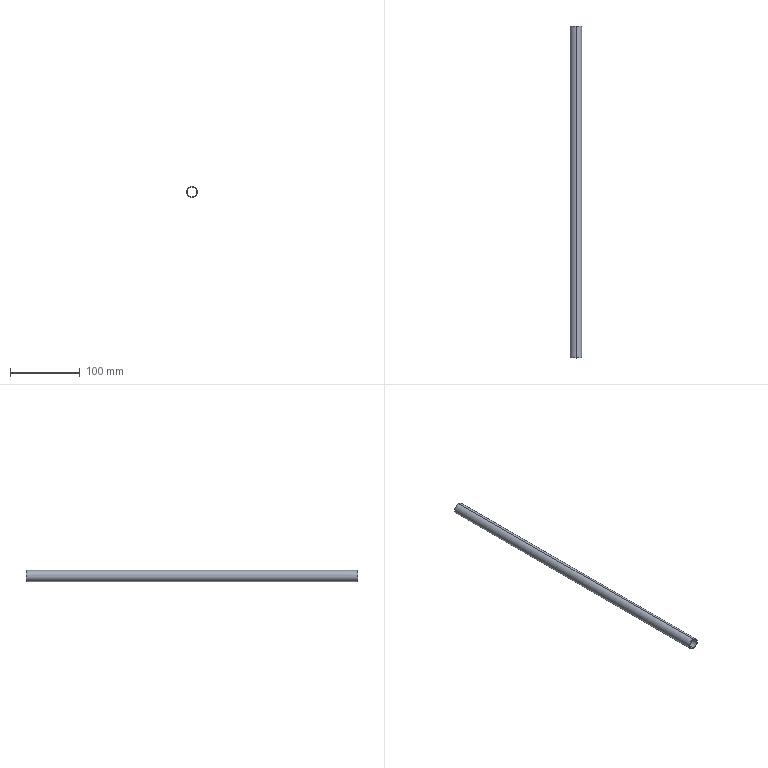Part | SolidWorks | features ExtruThin 1 | 1 solid | 6 faces | box 16 x 475 x 16 mm | volume 22384 mm3 | cylinder 4 | plane 2 | commonest cylinder face diameters 14 x2 16 x2
STEP:
#1=CARTESIAN_POINT('',(0.,475.,-7.));
#2=VERTEX_POINT('',#1);
#3=CARTESIAN_POINT('',(0.,475.,7.));
#4=VERTEX_POINT('',#3);
#5=CARTESIAN_POINT('',(0.,475.,0.));
#6=DIRECTION('',(0.,1.,0.));
#7=DIRECTION('',(1.,0.,0.));
#8=AXIS2_PLACEMENT_3D('',#5,#6,#7);
#9=CIRCLE('',#8,7.);
#10=EDGE_CURVE('',#2,#4,#9,.T.);
#11=ORIENTED_EDGE('',*,*,#10,.T.);
#12=CARTESIAN_POINT('',(0.,0.,7.));
#13=VERTEX_POINT('',#12);
#14=CARTESIAN_POINT('',(0.,475.,7.));
#15=DIRECTION('',(0.,-1.,0.));
#16=VECTOR('',#15,1000.);
#17=LINE('',#14,#16);
#18=EDGE_CURVE('',#4,#13,#17,.T.);
#19=ORIENTED_EDGE('',*,*,#18,.T.);
#20=CARTESIAN_POINT('',(0.,0.,-7.));
#21=VERTEX_POINT('',#20);
#22=CARTESIAN_POINT('',(0.,0.,0.));
#23=DIRECTION('',(0.,1.,0.));
#24=DIRECTION('',(1.,0.,0.));
#25=AXIS2_PLACEMENT_3D('',#22,#23,#24);
#26=CIRCLE('',#25,7.);
#27=EDGE_CURVE('',#21,#13,#26,.T.);
#28=ORIENTED_EDGE('',*,*,#27,.F.);
#29=CARTESIAN_POINT('',(0.,475.,-7.));
#30=DIRECTION('',(0.,-1.,0.));
#31=VECTOR('',#30,1000.);
#32=LINE('',#29,#31);
#33=EDGE_CURVE('',#2,#21,#32,.T.);
#34=ORIENTED_EDGE('',*,*,#33,.F.);
#35=EDGE_LOOP('',(#11,#19,#28,#34));
#36=FACE_OUTER_BOUND('',#35,.T.);
#37=CARTESIAN_POINT('',(0.,475.,0.));
#38=DIRECTION('',(0.,-1.,0.));
#39=DIRECTION('',(0.,0.,-1.));
#40=AXIS2_PLACEMENT_3D('',#37,#38,#39);
#41=CYLINDRICAL_SURFACE('',#40,7.);
#42=ADVANCED_FACE('',(#36),#41,.F.);
#43=CARTESIAN_POINT('',(0.,475.,8.));
#44=VERTEX_POINT('',#43);
#45=CARTESIAN_POINT('',(0.,475.,-8.));
#46=VERTEX_POINT('',#45);
#47=CARTESIAN_POINT('',(0.,475.,0.));
#48=DIRECTION('',(0.,1.,0.));
#49=DIRECTION('',(0.,0.,1.));
#50=AXIS2_PLACEMENT_3D('',#47,#48,#49);
#51=CIRCLE('',#50,8.);
#52=EDGE_CURVE('',#44,#46,#51,.T.);
#53=ORIENTED_EDGE('',*,*,#52,.F.);
#54=CARTESIAN_POINT('',(0.,0.,8.));
#55=VERTEX_POINT('',#54);
#56=CARTESIAN_POINT('',(0.,475.,8.));
#57=DIRECTION('',(0.,-1.,0.));
#58=VECTOR('',#57,1000.);
#59=LINE('',#56,#58);
#60=EDGE_CURVE('',#44,#55,#59,.T.);
#61=ORIENTED_EDGE('',*,*,#60,.T.);
#62=CARTESIAN_POINT('',(0.,0.,-8.));
#63=VERTEX_POINT('',#62);
#64=CARTESIAN_POINT('',(0.,0.,0.));
#65=DIRECTION('',(0.,1.,0.));
#66=DIRECTION('',(0.,0.,1.));
#67=AXIS2_PLACEMENT_3D('',#64,#65,#66);
#68=CIRCLE('',#67,8.);
#69=EDGE_CURVE('',#55,#63,#68,.T.);
#70=ORIENTED_EDGE('',*,*,#69,.T.);
#71=CARTESIAN_POINT('',(0.,475.,-8.));
#72=DIRECTION('',(0.,-1.,0.));
#73=VECTOR('',#72,1000.);
#74=LINE('',#71,#73);
#75=EDGE_CURVE('',#46,#63,#74,.T.);
#76=ORIENTED_EDGE('',*,*,#75,.F.);
#77=EDGE_LOOP('',(#53,#61,#70,#76));
#78=FACE_OUTER_BOUND('',#77,.T.);
#79=CARTESIAN_POINT('',(0.,475.,0.));
#80=DIRECTION('',(0.,-1.,0.));
#81=DIRECTION('',(0.,0.,-1.));
#82=AXIS2_PLACEMENT_3D('',#79,#80,#81);
#83=CYLINDRICAL_SURFACE('',#82,8.);
#84=ADVANCED_FACE('',(#78),#83,.T.);
#85=CARTESIAN_POINT('',(0.,475.,0.));
#86=DIRECTION('',(0.,1.,0.));
#87=DIRECTION('',(0.,0.,1.));
#88=AXIS2_PLACEMENT_3D('',#85,#86,#87);
#89=CIRCLE('',#88,8.);
#90=EDGE_CURVE('',#46,#44,#89,.T.);
#91=ORIENTED_EDGE('',*,*,#90,.T.);
#92=ORIENTED_EDGE('',*,*,#52,.T.);
#93=EDGE_LOOP('',(#91,#92));
#94=FACE_OUTER_BOUND('',#93,.T.);
#95=ORIENTED_EDGE('',*,*,#10,.F.);
#96=CARTESIAN_POINT('',(0.,475.,0.));
#97=DIRECTION('',(0.,1.,0.));
#98=DIRECTION('',(1.,0.,0.));
#99=AXIS2_PLACEMENT_3D('',#96,#97,#98);
#100=CIRCLE('',#99,7.);
#101=EDGE_CURVE('',#4,#2,#100,.T.);
#102=ORIENTED_EDGE('',*,*,#101,.F.);
#103=EDGE_LOOP('',(#95,#102));
#104=FACE_BOUND('',#103,.T.);
#105=CARTESIAN_POINT('',(0.,475.,0.));
#106=DIRECTION('',(0.,1.,0.));
#107=DIRECTION('',(0.,0.,1.));
#108=AXIS2_PLACEMENT_3D('',#105,#106,#107);
#109=PLANE('',#108);
#110=ADVANCED_FACE('',(#94,#104),#109,.T.);
#111=CARTESIAN_POINT('',(0.,0.,0.));
#112=DIRECTION('',(0.,1.,0.));
#113=DIRECTION('',(0.,0.,1.));
#114=AXIS2_PLACEMENT_3D('',#111,#112,#113);
#115=CIRCLE('',#114,8.);
#116=EDGE_CURVE('',#63,#55,#115,.T.);
#117=ORIENTED_EDGE('',*,*,#116,.F.);
#118=ORIENTED_EDGE('',*,*,#69,.F.);
#119=EDGE_LOOP('',(#117,#118));
#120=FACE_OUTER_BOUND('',#119,.T.);
#121=ORIENTED_EDGE('',*,*,#27,.T.);
#122=CARTESIAN_POINT('',(0.,0.,0.));
#123=DIRECTION('',(0.,1.,0.));
#124=DIRECTION('',(1.,0.,0.));
#125=AXIS2_PLACEMENT_3D('',#122,#123,#124);
#126=CIRCLE('',#125,7.);
#127=EDGE_CURVE('',#13,#21,#126,.T.);
#128=ORIENTED_EDGE('',*,*,#127,.T.);
#129=EDGE_LOOP('',(#121,#128));
#130=FACE_BOUND('',#129,.T.);
#131=CARTESIAN_POINT('',(0.,0.,0.));
#132=DIRECTION('',(0.,1.,0.));
#133=DIRECTION('',(0.,0.,1.));
#134=AXIS2_PLACEMENT_3D('',#131,#132,#133);
#135=PLANE('',#134);
#136=ADVANCED_FACE('',(#120,#130),#135,.F.);
#137=ORIENTED_EDGE('',*,*,#60,.F.);
#138=ORIENTED_EDGE('',*,*,#90,.F.);
#139=ORIENTED_EDGE('',*,*,#75,.T.);
#140=ORIENTED_EDGE('',*,*,#116,.T.);
#141=EDGE_LOOP('',(#137,#138,#139,#140));
#142=FACE_OUTER_BOUND('',#141,.T.);
#143=CARTESIAN_POINT('',(0.,475.,0.));
#144=DIRECTION('',(0.,-1.,0.));
#145=DIRECTION('',(0.,0.,-1.));
#146=AXIS2_PLACEMENT_3D('',#143,#144,#145);
#147=CYLINDRICAL_SURFACE('',#146,8.);
#148=ADVANCED_FACE('',(#142),#147,.T.);
#149=ORIENTED_EDGE('',*,*,#18,.F.);
#150=ORIENTED_EDGE('',*,*,#101,.T.);
#151=ORIENTED_EDGE('',*,*,#33,.T.);
#152=ORIENTED_EDGE('',*,*,#127,.F.);
#153=EDGE_LOOP('',(#149,#150,#151,#152));
#154=FACE_OUTER_BOUND('',#153,.T.);
#155=CARTESIAN_POINT('',(0.,475.,0.));
#156=DIRECTION('',(0.,-1.,0.));
#157=DIRECTION('',(0.,0.,-1.));
#158=AXIS2_PLACEMENT_3D('',#155,#156,#157);
#159=CYLINDRICAL_SURFACE('',#158,7.);
#160=ADVANCED_FACE('',(#154),#159,.F.);
#161=CLOSED_SHELL('',(#42,#84,#110,#136,#148,#160));
#162=MANIFOLD_SOLID_BREP('',#161);
#163=CARTESIAN_POINT('',(0.,0.,0.));
#164=DIRECTION('',(0.,0.,1.));
#165=DIRECTION('',(1.,0.,0.));
#166=AXIS2_PLACEMENT_3D('',#163,#164,#165);
#167=(LENGTH_UNIT()NAMED_UNIT(*)SI_UNIT(.MILLI.,.METRE.));
#168=UNCERTAINTY_MEASURE_WITH_UNIT(LENGTH_MEASURE(0.00001),#167,'','');
#169=(NAMED_UNIT(*)PLANE_ANGLE_UNIT()SI_UNIT($,.RADIAN.));
#170=(NAMED_UNIT(*)SI_UNIT($,.STERADIAN.)SOLID_ANGLE_UNIT());
#171=(GEOMETRIC_REPRESENTATION_CONTEXT(3)GLOBAL_UNCERTAINTY_ASSIGNED_CONTEXT((#168))GLOBAL_UNIT_ASSIGNED_CONTEXT((#167,#169,#170))REPRESENTATION_CONTEXT('',''));
#172=ADVANCED_BREP_SHAPE_REPRESENTATION('',(#162,#166),#171);